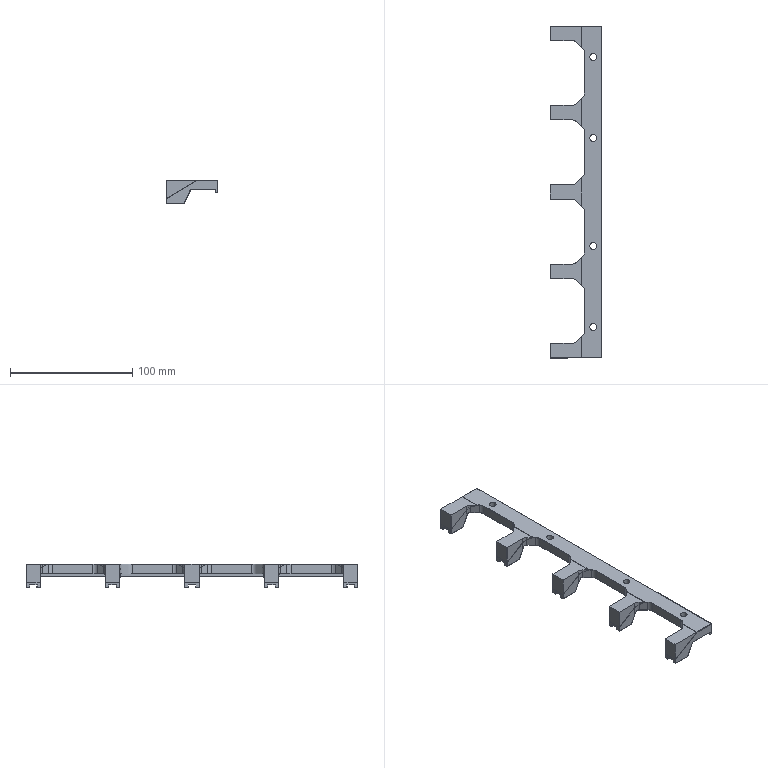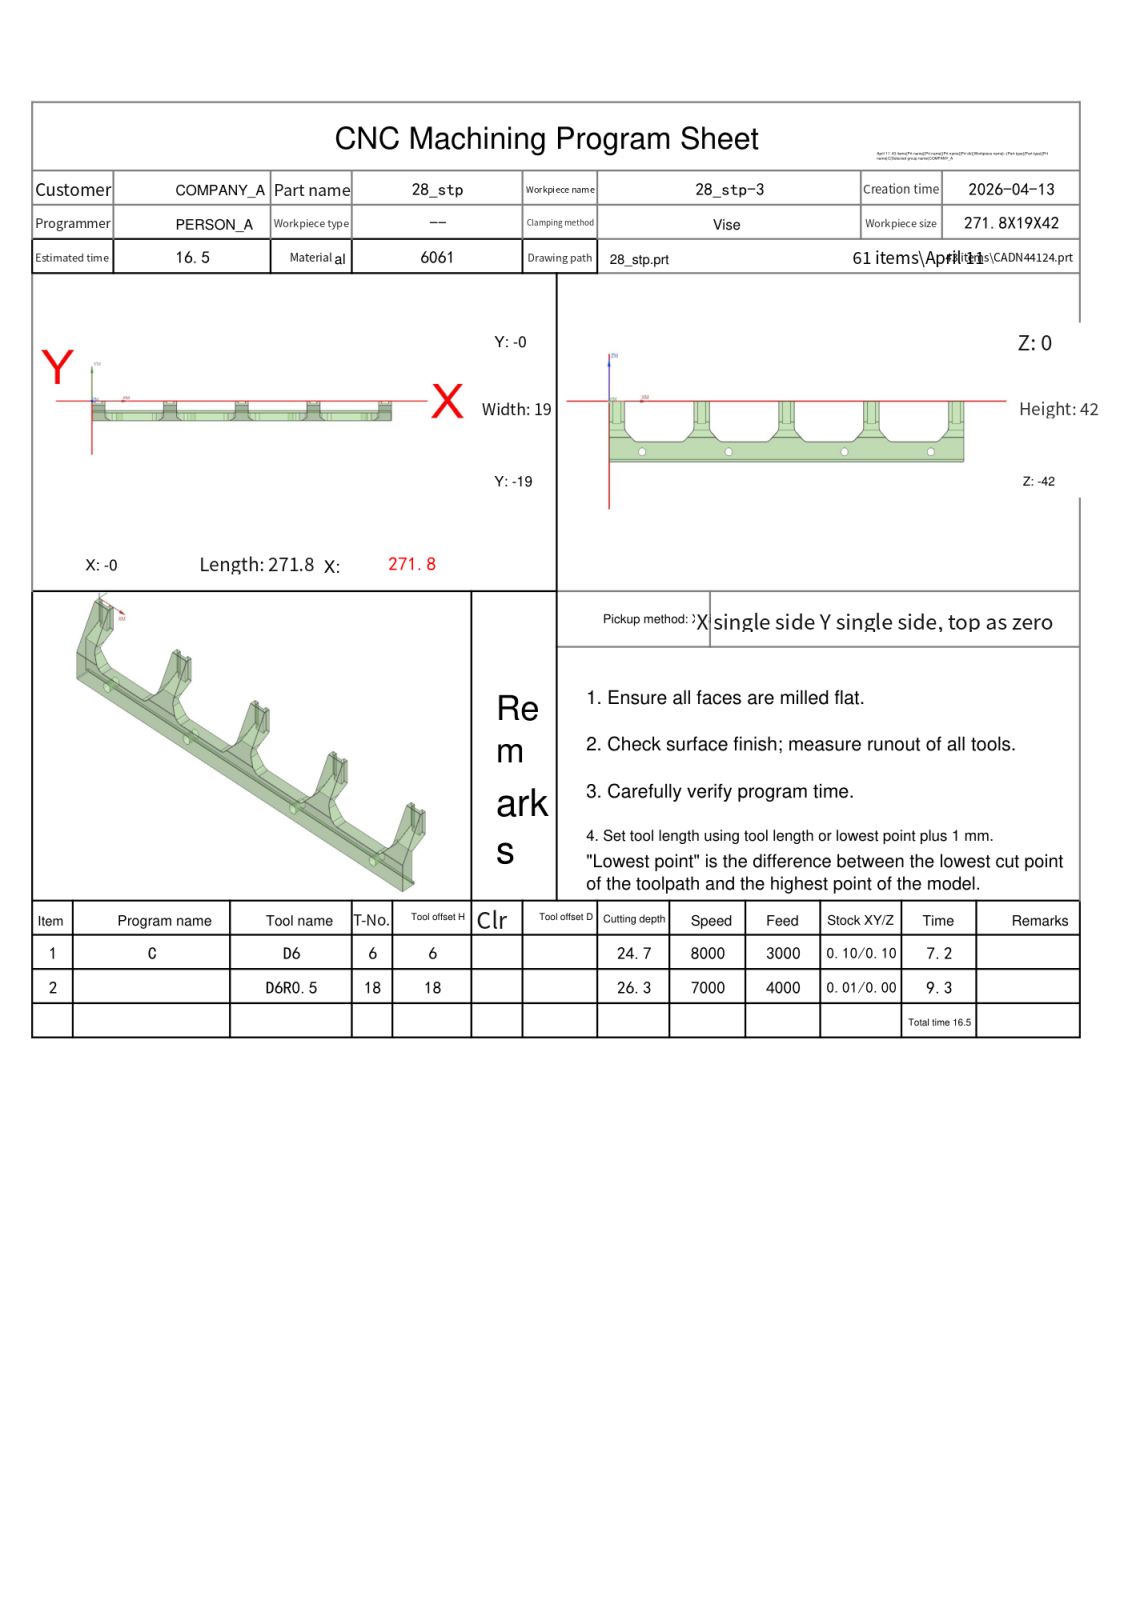NC program | NX | posted by the shop | part box 42 x 271.8 x 19 mm
Lines 8981 to 10169 of 25484:
N2 T18 M06
(D6R0.5  D=6. R=0.5 H=18 ce=0.01 di=0.00)
G00 G90 G54 X264.168 Y-6.651 M03 S7000
G43 H18 Z11.1
M08
Z1.113
G01 Z.613 F4000.
X259.69 Y-5.416
X258.972 Y-5.218
X258.804 Y-5.139
X258.651 Y-5.118 Z.595
X258.511 Y-5.071 Z.577
X258.381 Y-5.011 Z.559
G03 X260.049 Y-5.545 I1.668 J2.336
G01 X260.103
X260.241 Y-5.588 Z.533
X260.379 Y-5.628 Z.507
G02 X260.097 Y-5.641 I-.282 J3.036
X258.218 Y-4.993 I0.0 J3.049
G00 Z11.1
X17.341 Y-3.657
Z1.113
G01 Z.613
X12.763 Y-5.211
X12.436 Y-5.322
X12.366 Y-5.334
X12.217 Y-5.404 Z.599
X12.064 Y-5.461 Z.586
X11.91 Y-5.499 Z.572
X11.756 Y-5.527 Z.559
G03 X13.39 Y-5.009 I-.03 J2.93
G01 X13.505 Y-5.001 Z.533
X13.608 Y-4.976 Z.507
G02 X11.623 Y-5.635 I-1.985 J2.665
X11.423 Y-5.629 I0.0 J3.323
G00 Z11.1
X4.846 Y-5.95
Z1.113
G01 Z.613
X-.217 Y-5.414
G02 X-1.126 Y-5.134 I.26 J2.453
G01 X-1.278 Y-5.109 Z.595
X-1.417 Y-5.061 Z.577
X-1.548 Y-5.001 Z.559
G03 X.124 Y-5.546 I1.672 J2.294
G01 X.203 Y-5.545
X.325 Y-5.577 Z.542
X.447 Y-5.604 Z.524
X.569 Y-5.628 Z.507
G02 X.229 Y-5.646 I-.339 J3.2
X-1.737 Y-4.975 I0.0 J3.218
G01 X-1.81 Y-4.996 Z.458
G03 X.183 Y-5.717 I1.996 J2.4
G01 X2.073 Y-5.719
X11.093 Y-5.718
X11.682 Y-5.717
G03 X13.703 Y-4.991 I-.011 J3.206
G01 X13.771 Y-5.013 Z.409
G02 X11.657 Y-5.805 I-2.115 J2.43
G01 X2.073 Y-5.806
X.205 Y-5.802
G02 X-1.878 Y-5.016 I.007 J3.172
G01 X-1.946 Y-5.037 Z.359
G03 X.251 Y-5.887 I2.208 J2.441
G01 X2.073 Y-5.893
X11.642 Y-5.892
G03 X13.84 Y-5.036 I0.0 J3.253
G01 X13.915 Y-5.052 Z.31
G02 X11.62 Y-5.979 I-2.295 J2.379
G01 X2.073 Y-5.98
X.685 Y-5.975
X.228 Y-5.972
G02 X-1.701 Y-5.303 I.019 J3.169
G01 X-2.015 Y-5.059
X-2.085 Y-5.083 Z.261
X-1.396 Y-5.59
G03 X.309 Y-6.06 I1.705 J2.858
G01 X.338
X2.073 Y-6.067
X11.44 Y-6.066
X11.788 Y-6.06
G03 X13.302 Y-5.588 I-.055 J2.843
X13.993 Y-5.064 I-3.716 J5.62
G01 X14.071 Y-5.077 Z.212
X13.453 Y-5.555
G02 X11.704 Y-6.154 I-1.749 J2.258
G01 X1.379 Y-6.153
X.26 Y-6.148
G02 X-1.35 Y-5.687 I.014 J3.095
X-2.171 Y-5.084 I3.325 J5.394
G01 X-2.259 Y-5.085 Z.162
X-1.563 Y-5.618
G03 X.247 Y-6.236 I1.824 J2.383
G01 X1.379 Y-6.241
X11.667
G03 X13.528 Y-5.587 I0.0 J2.978
G01 X14.15 Y-5.09
X14.239 Y-5.093 Z.113
X14.216 Y-5.114
X13.522 Y-5.669
G02 X11.787 Y-6.323 I-1.874 J2.344
G01 X11.44 Y-6.328
X1.379 Y-6.329
X.257 Y-6.324
G02 X-1.603 Y-5.674 I.013 J3.024
G01 X-2.347 Y-5.087
X-2.436 Y-5.09 Z.064
X-1.563 Y-5.778
G03 X.256 Y-6.412 I1.829 J2.321
G01 X1.379 Y-6.416
X11.648 Y-6.414
X11.762 Y-6.411
G03 X13.295 Y-5.902 I-.064 J2.755
X14.367 Y-5.051 I-7.464 J10.497
G01 X14.491 Y-5.012 Z.017
G02 X13.354 Y-5.937 I-11.479 J12.943
X11.721 Y-6.496 I-1.685 J2.259
G01 X11.648 Y-6.497
X.261 Y-6.496
G02 X-1.558 Y-5.856 I0.0 J2.905
G01 X-2.437 Y-5.149
X-2.578 Y-5.025
X-2.677 Y-4.98 Z-.016
G03 X-2.195 Y-5.394 I6.378 J6.933
G01 X-1.532 Y-5.926
G03 X.256 Y-6.555 I1.789 J2.229
G01 X11.579 Y-6.556
X11.642 Y-6.557
G03 X13.315 Y-6.02 I0.0 J2.876
X14.576 Y-4.98 I-10.632 J14.176
G01 X14.637 Y-4.951 Z-.053
G02 X13.307 Y-6.082 I-8.368 J8.492
X11.718 Y-6.62 I-1.66 J2.287
G01 X.252
G02 X-1.506 Y-6.009 I.009 J2.86
G01 X-2.343 Y-5.316
G02 X-2.761 Y-4.93 I3.319 J4.01
G01 X-2.803 Y-4.925 Z-.098
G03 X-2.01 Y-5.666 I5.054 J4.614
G01 X-1.743 Y-5.882
X-1.596 Y-6.009
G03 X.256 Y-6.701 I1.875 J2.193
G01 X11.646
G03 X13.257 Y-6.185 I0.0 J2.771
X14.709 Y-4.915 I-5.715 J7.996
G01 X14.776 Y-4.872 Z-.145
G02 X13.817 Y-5.816 I-5.844 J4.98
G01 X13.479 Y-6.095
G02 X11.624 Y-6.785 I-1.911 J2.3
G01 X.276
G02 X-1.396 Y-6.231 I.005 J2.817
G01 X-1.679 Y-6.009
G02 X-2.826 Y-4.932 I4.857 J6.325
G01 X-2.849 Y-4.938 Z-.198
G03 X-1.338 Y-6.353 I6.547 J5.482
X.284 Y-6.869 I1.632 J2.321
G01 X11.613
G03 X13.453 Y-6.191 I-.023 J2.901
G01 X13.578 Y-6.088
G03 X14.85 Y-4.822 I-5.324 J6.62
G01 X14.91 Y-4.794 Z-.261
X14.216 Y-5.584
X14.136 Y-5.666
X13.63 Y-6.136
X13.462 Y-6.275
G02 X11.614 Y-6.938 I-1.848 J2.241
G01 X.282
G02 X-1.534 Y-6.295 I0.0 J2.886
X-2.877 Y-4.945 I5.583 J6.895
G01 X-2.907 Y-4.952 Z-.329
G03 X-1.963 Y-6.009 I14.585 J12.07
X.283 Y-6.99 I2.25 J2.09
G01 X11.614
G03 X13.861 Y-6.009 I-.001 J3.066
X14.911 Y-4.833 I-15.381 J14.784
G01 X14.912 Y-4.878 Z-.407
G02 X13.869 Y-6.076 I-37.077 J31.237
X11.691 Y-7.037 I-2.178 J1.987
G01 X11.684
X.209
G02 X-1.95 Y-6.095 I0.0 J2.948
G01 X-2.09 Y-5.945
X-2.94 Y-4.96
X-2.976 Y-4.969 Z-.488
X-2.229 Y-5.841
X-2.09 Y-6.003
G03 X.2 Y-7.086 I2.304 J1.908
G01 X11.7
G03 X13.983 Y-6.011 I-.028 J3.02
G01 X14.129 Y-5.841
X14.913 Y-4.926
X14.914 Y-4.974 Z-.572
X14.159 Y-5.856
X13.959 Y-6.089
G02 X11.7 Y-7.136 I-2.268 J1.933
G01 X.2
G02 X-2.059 Y-6.089 I.009 J2.98
G01 X-2.259 Y-5.856
X-3.012 Y-4.978
X-3.014 Y-5.025 Z-.657
X-2.259 Y-5.907
X-2.059 Y-6.141
G03 X.2 Y-7.188 I2.268 J1.933
G01 X11.7
G03 X13.959 Y-6.141 I-.009 J2.98
G01 X14.159 Y-5.907
X14.915 Y-5.025
Y-5.076 Z-.743
X14.159 Y-5.959
X13.959 Y-6.192
G02 X11.7 Y-7.239 I-2.268 J1.933
G01 X.2
G02 X-2.059 Y-6.192 I.009 J2.98
G01 X-2.259 Y-5.959
X-3.014 Y-5.075
Y-5.125 Z-.829
X-2.259 Y-6.01
X-2.059 Y-6.244
G03 X.2 Y-7.29 I2.268 J1.933
G01 X11.7
G03 X13.959 Y-6.244 I-.009 J2.98
G01 X14.159 Y-6.01
X14.916 Y-5.127
Y-5.178 Z-.915
X14.159 Y-6.062
X13.959 Y-6.295
G02 X11.7 Y-7.342 I-2.268 J1.933
G01 X.2
G02 X-2.059 Y-6.295 I.009 J2.98
G01 X-2.259 Y-6.062
X-2.893 Y-5.322
X-3.014 Y-5.177
X-3.015 Y-5.228 Z-1.
X-2.937 Y-5.322
X-2.259 Y-6.113
X-2.059 Y-6.346
G03 X.2 Y-7.393 I2.268 J1.933
G01 X11.7
G03 X13.959 Y-6.346 I-.009 J2.98
G01 X14.159 Y-6.113
X14.917 Y-5.229
Y-5.28 Z-1.086
X14.159 Y-6.165
X13.959 Y-6.398
G02 X11.7 Y-7.445 I-2.268 J1.933
G01 X.2
G02 X-2.059 Y-6.398 I.009 J2.98
G01 X-2.259 Y-6.165
X-2.982 Y-5.322
X-3.017 Y-5.279
X-3.018 Y-5.331 Z-1.172
X-2.259 Y-6.216
X-2.059 Y-6.449
G03 X.2 Y-7.496 I2.268 J1.933
G01 X11.7
G03 X13.959 Y-6.449 I-.009 J2.98
G01 X14.159 Y-6.216
X14.918 Y-5.331
Y-5.382 Z-1.258
X14.159 Y-6.268
X13.959 Y-6.501
G02 X11.7 Y-7.548 I-2.268 J1.933
G01 X.2
G02 X-2.059 Y-6.501 I.009 J2.98
G01 X-2.259 Y-6.268
X-3.017 Y-5.381
Y-5.431 Z-1.343
X-2.259 Y-6.319
X-2.059 Y-6.552
G03 X.2 Y-7.599 I2.268 J1.933
G01 X11.7
G03 X13.959 Y-6.552 I-.009 J2.98
G01 X14.159 Y-6.319
X14.918 Y-5.433
X14.919 Y-5.483 Z-1.429
X14.159 Y-6.37
X13.959 Y-6.604
G02 X11.7 Y-7.651 I-2.268 J1.933
G01 X.2
G02 X-2.059 Y-6.604 I.009 J2.98
G01 X-2.259 Y-6.37
X-3.017 Y-5.482
X-3.018 Y-5.533 Z-1.515
X-2.908 Y-5.666
X-2.259 Y-6.422
X-2.059 Y-6.655
G03 X.2 Y-7.702 I2.268 J1.933
G01 X11.7
G03 X13.959 Y-6.655 I-.009 J2.98
G01 X14.159 Y-6.422
X14.919 Y-5.534
X14.92 Y-5.585 Z-1.601
X14.159 Y-6.473
X13.959 Y-6.707
G02 X11.7 Y-7.754 I-2.268 J1.933
G01 X.2
G02 X-2.059 Y-6.707 I.009 J2.98
G01 X-2.259 Y-6.473
X-2.952 Y-5.666
X-3.019 Y-5.585
X-3.02 Y-5.636 Z-1.686
X-2.996 Y-5.666
X-2.259 Y-6.525
X-2.059 Y-6.758
G03 X.2 Y-7.805 I2.268 J1.933
G01 X11.7
G03 X13.959 Y-6.758 I-.009 J2.98
G01 X14.159 Y-6.525
X14.909 Y-5.65
X14.92 Y-5.636
X14.921 Y-5.687 Z-1.772
X14.159 Y-6.576
X13.959 Y-6.81
G02 X11.7 Y-7.856 I-2.268 J1.933
G01 X.2
G02 X-2.059 Y-6.81 I.009 J2.98
G01 X-2.259 Y-6.576
X-3.021 Y-5.687
X-3.02 Y-5.737 Z-1.858
X-2.259 Y-6.628
X-2.059 Y-6.861
G03 X.2 Y-7.908 I2.268 J1.933
G01 X11.7
G03 X13.959 Y-6.861 I-.009 J2.98
G01 X14.159 Y-6.628
X14.921 Y-5.738
Y-5.789 Z-1.944
X14.159 Y-6.679
X13.959 Y-6.912
G02 X11.7 Y-7.959 I-2.268 J1.933
G01 X.2
G02 X-2.059 Y-6.912 I.009 J2.98
G01 X-2.259 Y-6.679
X-3.02 Y-5.788
Y-5.839 Z-2.029
X-2.878 Y-6.009
X-2.259 Y-6.731
X-2.059 Y-6.964
G03 X.2 Y-8.011 I2.268 J1.933
G01 X11.7
G03 X13.959 Y-6.964 I-.009 J2.98
G01 X14.159 Y-6.731
X14.922 Y-5.84
Y-5.891 Z-2.115
X14.159 Y-6.782
X13.959 Y-7.015
G02 X11.7 Y-8.062 I-2.268 J1.933
G01 X.2
G02 X-2.059 Y-7.015 I.009 J2.98
G01 X-2.259 Y-6.782
X-2.922 Y-6.009
X-3.021 Y-5.89
X-3.022 Y-5.941 Z-2.201
X-2.966 Y-6.009
X-2.259 Y-6.833
X-2.059 Y-7.067
G03 X.2 Y-8.114 I2.268 J1.933
G01 X11.7
G03 X13.959 Y-7.067 I-.009 J2.98
G01 X14.159 Y-6.833
X14.909 Y-5.959
X14.922 Y-5.941
X14.923 Y-5.992 Z-2.287
X14.91 Y-6.009
X14.159 Y-6.885
X13.959 Y-7.118
G02 X11.7 Y-8.165 I-2.268 J1.933
G01 X.2
G02 X-2.059 Y-7.118 I.009 J2.98
G01 X-2.259 Y-6.885
X-3.023 Y-5.993
Y-6.044 Z-2.372
X-2.259 Y-6.936
X-2.059 Y-7.17
G03 X.2 Y-8.217 I2.268 J1.933
G01 X11.7
G03 X13.959 Y-7.17 I-.009 J2.98
G01 X14.159 Y-6.936
X14.924 Y-6.044
Y-6.095 Z-2.458
X14.159 Y-6.988
X13.959 Y-7.221
G02 X11.7 Y-8.268 I-2.268 J1.933
G01 X.2
G02 X-2.059 Y-7.221 I.009 J2.98
G01 X-2.259 Y-6.988
X-3.023 Y-6.094
Y-6.145 Z-2.544
X-2.259 Y-7.039
X-2.059 Y-7.273
G03 X.2 Y-8.319 I2.268 J1.933
G01 X11.7
G03 X13.959 Y-7.273 I-.009 J2.98
G01 X14.159 Y-7.039
X14.924 Y-6.146
X14.925 Y-6.197 Z-2.63
X14.159 Y-7.091
X13.959 Y-7.324
G02 X11.7 Y-8.371 I-2.268 J1.933
G01 X.2
G02 X-2.059 Y-7.324 I.009 J2.98
G01 X-2.259 Y-7.091
X-2.892 Y-6.353
X-3.023 Y-6.196
X-3.024 Y-6.247 Z-2.715
X-2.936 Y-6.353
X-2.259 Y-7.142
X-2.059 Y-7.375
G03 X.2 Y-8.422 I2.268 J1.933
G01 X11.7
G03 X13.959 Y-7.375 I-.009 J2.98
G01 X14.159 Y-7.142
X14.909 Y-6.267
X14.925 Y-6.247
Y-6.298 Z-2.801
X14.909 Y-6.319
X14.159 Y-7.194
X13.959 Y-7.427
G02 X11.7 Y-8.474 I-2.268 J1.933
G01 X.2
G02 X-2.059 Y-7.427 I.009 J2.98
G01 X-2.259 Y-7.194
X-2.98 Y-6.353
X-3.025 Y-6.299
X-3.026 Y-6.351 Z-2.887
X-2.259 Y-7.245
X-2.059 Y-7.478
G03 X.2 Y-8.525 I2.268 J1.933
G01 X11.7
G03 X13.959 Y-7.478 I-.009 J2.98
G01 X14.159 Y-7.245
X14.927 Y-6.35
X14.926 Y-6.401 Z-2.973
X14.159 Y-7.297
X13.959 Y-7.53
G02 X11.7 Y-8.577 I-2.268 J1.933
G01 X.2
G02 X-2.059 Y-7.53 I.009 J2.98
G01 X-2.259 Y-7.297
X-3.026 Y-6.401
X-3.025 Y-6.451 Z-3.058
X-2.259 Y-7.348
X-2.059 Y-7.581
G03 X.2 Y-8.628 I2.268 J1.933
G01 X11.7
G03 X13.959 Y-7.581 I-.009 J2.98
G01 X14.159 Y-7.348
X14.927 Y-6.452
Y-6.503 Z-3.144
X14.909 Y-6.525
X14.159 Y-7.399
X13.959 Y-7.633
G02 X11.7 Y-8.68 I-2.268 J1.933
G01 X.2
G02 X-2.059 Y-7.633 I.009 J2.98
G01 X-2.259 Y-7.399
X-3.025 Y-6.502
X-3.026 Y-6.553 Z-3.23
X-2.906 Y-6.696
X-2.259 Y-7.451
X-2.059 Y-7.684
G03 X.2 Y-8.731 I2.268 J1.933
G01 X11.7
G03 X13.959 Y-7.684 I-.009 J2.98
G01 X14.159 Y-7.451
X14.909 Y-6.576
X14.927 Y-6.554
Y-6.605 Z-3.316
X14.909 Y-6.627
X14.159 Y-7.502
X13.959 Y-7.736
G02 X11.7 Y-8.783 I-2.268 J1.933
G01 X.2
G02 X-2.059 Y-7.736 I.009 J2.98
G01 X-2.259 Y-7.502
X-2.95 Y-6.696
X-3.027 Y-6.605
X-3.028 Y-6.656 Z-3.401
X-2.994 Y-6.696
X-2.259 Y-7.554
X-2.059 Y-7.787
G03 X.2 Y-8.834 I2.268 J1.933
G01 X11.7
G03 X13.959 Y-7.787 I-.009 J2.98
G01 X14.159 Y-7.554
X14.909 Y-6.679
X14.927 Y-6.656
X14.929 Y-6.707 Z-3.487
X14.159 Y-7.605
X13.959 Y-7.839
G02 X11.7 Y-8.885 I-2.268 J1.933
G01 X.2
G02 X-2.059 Y-7.839 I.009 J2.98
G01 X-2.259 Y-7.605
X-3.028 Y-6.708
Y-6.758 Z-3.573
X-2.259 Y-7.657
X-2.059 Y-7.89
G03 X.2 Y-8.937 I2.268 J1.933
G01 X11.7
G03 X13.959 Y-7.89 I-.009 J2.98
G01 X14.159 Y-7.657
X14.909 Y-6.782
X14.928 Y-6.758
X14.929 Y-6.809 Z-3.659
X14.909 Y-6.833
X14.159 Y-7.708
X13.959 Y-7.941
G02 X11.7 Y-8.988 I-2.268 J1.933
G01 X.2
G02 X-2.059 Y-7.941 I.009 J2.98
G01 X-2.259 Y-7.708
X-3.027 Y-6.808
X-3.028 Y-6.86 Z-3.744
X-2.876 Y-7.04
X-2.259 Y-7.76
X-2.059 Y-7.993
G03 X.2 Y-9.04 I2.268 J1.933
G01 X11.7
G03 X13.959 Y-7.993 I-.009 J2.98
G01 X14.159 Y-7.76
X14.909 Y-6.885
X14.929 Y-6.86
Y-6.911 Z-3.83
X14.909 Y-6.936
X14.159 Y-7.811
X13.959 Y-8.044
G02 X11.7 Y-9.091 I-2.268 J1.933
G01 X.2
G02 X-2.059 Y-8.044 I.009 J2.98
G01 X-2.259 Y-7.811
X-2.92 Y-7.04
X-3.028 Y-6.911
X-3.029 Y-6.962 Z-3.916
X-2.965 Y-7.04
X-2.259 Y-7.862
X-2.059 Y-8.096
G03 X.2 Y-9.143 I2.268 J1.933
G01 X11.7
G03 X13.959 Y-8.096 I-.009 J2.98
G01 X14.159 Y-7.862
X14.909 Y-6.988
X14.929 Y-6.962
Y-7.013 Z-4.002
X14.909 Y-7.039
X14.159 Y-7.914
X13.959 Y-8.147
G02 X11.7 Y-9.194 I-2.268 J1.933
G01 X.2
G02 X-2.059 Y-8.147 I.009 J2.98
G01 X-2.259 Y-7.914
X-3.009 Y-7.04
X-3.03 Y-7.014
Y-7.065 Z-4.087
X-2.259 Y-7.965
X-2.059 Y-8.199
G03 X.2 Y-9.246 I2.268 J1.933
G01 X11.7
G03 X13.959 Y-8.199 I-.009 J2.98
G01 X14.159 Y-7.965
X14.909 Y-7.091
X14.931 Y-7.065
Y-7.116 Z-4.173
X14.909 Y-7.142
X14.159 Y-8.017
X13.959 Y-8.25
G02 X11.7 Y-9.297 I-2.268 J1.933
G01 X.2
G02 X-2.059 Y-8.25 I.009 J2.98
G01 X-2.259 Y-8.017
X-3.03 Y-7.116
X-3.029 Y-7.166 Z-4.259
X-2.259 Y-8.068
X-2.059 Y-8.302
G03 X.2 Y-9.348 I2.268 J1.933
G01 X11.7
G03 X13.959 Y-8.302 I-.009 J2.98
G01 X14.159 Y-8.068
X14.909 Y-7.193
X14.931 Y-7.167
Y-7.218 Z-4.345
X14.909 Y-7.245
X14.159 Y-8.12
X13.959 Y-8.353
G02 X11.7 Y-9.4 I-2.268 J1.933
G01 X.2
G02 X-2.059 Y-8.353 I.009 J2.98
G01 X-2.259 Y-8.12
X-2.891 Y-7.384
X-3.03 Y-7.218
Y-7.269 Z-4.43
X-2.935 Y-7.384
X-2.259 Y-8.171
X-2.059 Y-8.404
G03 X.2 Y-9.451 I2.268 J1.933
G01 X11.7
G03 X13.959 Y-8.404 I-.009 J2.98
G01 X14.159 Y-8.171
X14.909 Y-7.296
X14.931 Y-7.269
Y-7.32 Z-4.516
X14.909 Y-7.348
X14.159 Y-8.223
X13.959 Y-8.456
G02 X11.7 Y-9.503 I-2.268 J1.933
G01 X.2
G02 X-2.059 Y-8.456 I.009 J2.98
G01 X-2.259 Y-8.223
X-2.979 Y-7.384
X-3.031 Y-7.321
X-3.032 Y-7.372 Z-4.602
X-2.259 Y-8.274
X-2.059 Y-8.507
G03 X.2 Y-9.554 I2.268 J1.933
G01 X11.7
G03 X13.959 Y-8.507 I-.009 J2.98
G01 X14.159 Y-8.274
X14.923 Y-7.384
X14.932 Y-7.372
Y-7.423 Z-4.688
X14.909 Y-7.451
X14.159 Y-8.326
X13.959 Y-8.559
G02 X11.7 Y-9.606 I-2.268 J1.933
G01 X.2
G02 X-2.059 Y-8.559 I.009 J2.98
G01 X-2.259 Y-8.326
X-3.032 Y-7.423
X-3.031 Y-7.474 Z-4.773
X-2.259 Y-8.377
X-2.059 Y-8.61
G03 X.2 Y-9.657 I2.268 J1.933
G01 X11.7
G03 X13.959 Y-8.61 I-.009 J2.98
G01 X14.159 Y-8.377
X14.909 Y-7.502
X14.932 Y-7.474
Y-7.525 Z-4.859
X14.909 Y-7.554
X14.159 Y-8.428
X13.959 Y-8.662
G02 X11.7 Y-9.709 I-2.268 J1.933
G01 X.2
G02 X-2.059 Y-8.662 I.009 J2.98
G01 X-2.259 Y-8.428
X-3.031 Y-7.525
Y-7.576 Z-4.945
X-2.905 Y-7.727
X-2.259 Y-8.48
X-2.059 Y-8.713
G03 X.2 Y-9.76 I2.268 J1.933
G01 X11.7
G03 X13.959 Y-8.713 I-.009 J2.98
G01 X14.159 Y-8.48
X14.909 Y-7.605
X14.932 Y-7.576
Y-7.627 Z-5.031
X14.909 Y-7.656
X14.159 Y-8.531
X13.959 Y-8.765
G02 X11.7 Y-9.811 I-2.268 J1.933
G01 X.2
G02 X-2.059 Y-8.765 I.009 J2.98
G01 X-2.259 Y-8.531
X-2.949 Y-7.727
X-3.032 Y-7.628
Y-7.679 Z-5.116
X-2.993 Y-7.727
X-2.259 Y-8.583
X-2.059 Y-8.816
G03 X.2 Y-9.863 I2.268 J1.933
G01 X11.7
G03 X13.959 Y-8.816 I-.009 J2.98
G01 X14.159 Y-8.583
X14.909 Y-7.708
X14.932 Y-7.678
X14.934 Y-7.731 Z-5.202
X14.159 Y-8.634
X13.959 Y-8.868
G02 X11.7 Y-9.914 I-2.268 J1.933
G01 X.2
G02 X-2.059 Y-8.868 I.009 J2.98
G01 X-2.259 Y-8.634
X-3.033 Y-7.731
X-3.032 Y-7.782 Z-5.288
X-2.259 Y-8.686
X-2.059 Y-8.919
G03 X.2 Y-9.966 I2.268 J1.933
G01 X11.7
G03 X13.959 Y-8.919 I-.009 J2.98
G01 X14.159 Y-8.686
X14.909 Y-7.811
X14.933 Y-7.782
Y-7.833 Z-5.374
X14.909 Y-7.862
X14.159 Y-8.737
X13.959 Y-8.97
G02 X11.7 Y-10.017 I-2.268 J1.933
G01 X.2
G02 X-2.059 Y-8.97 I.009 J2.98
G01 X-2.259 Y-8.737
X-3.032 Y-7.832
Y-7.884 Z-5.459
X-2.259 Y-8.789
X-2.059 Y-9.022
G03 X.2 Y-10.069 I2.268 J1.933
G01 X11.7
G03 X13.959 Y-9.022 I-.009 J2.98
G01 X14.159 Y-8.789
X14.909 Y-7.914
X14.933 Y-7.884
Y-7.935 Z-5.545
X14.909 Y-7.965
X14.159 Y-8.84
X13.959 Y-9.073
G02 X11.7 Y-10.12 I-2.268 J1.933
G01 X.2
G02 X-2.059 Y-9.073 I.009 J2.98
G01 X-2.259 Y-8.84
X-2.919 Y-8.071
X-3.032 Y-7.935
X-3.033 Y-7.987 Z-5.631
X-2.963 Y-8.071
X-2.259 Y-8.891
X-2.059 Y-9.125
G03 X.2 Y-10.172 I2.268 J1.933
G01 X11.7
G03 X13.959 Y-9.125 I-.009 J2.98
G01 X14.159 Y-8.891
X14.909 Y-8.017
X14.933 Y-7.986
Y-8.037 Z-5.717
X14.909 Y-8.068
X14.159 Y-8.943
X13.959 Y-9.176
G02 X11.7 Y-10.223 I-2.268 J1.933
G01 X.2
G02 X-2.059 Y-9.176 I.009 J2.98
G01 X-2.259 Y-8.943
X-3.007 Y-8.071
X-3.034 Y-8.039
Y-8.09 Z-5.802
X-2.259 Y-8.994
X-2.059 Y-9.228
G03 X.2 Y-10.275 I2.268 J1.933
G01 X11.7
G03 X13.959 Y-9.228 I-.009 J2.98
G01 X14.159 Y-8.994
X14.934 Y-8.089
Y-8.141 Z-5.888
X14.909 Y-8.171
X14.159 Y-9.046
X13.959 Y-9.279
G02 X11.7 Y-10.326 I-2.268 J1.933
G01 X.2
G02 X-2.059 Y-9.279 I.009 J2.98
G01 X-2.259 Y-9.046
X-3.033 Y-8.141
Y-8.191 Z-5.974
X-2.259 Y-9.097
X-2.059 Y-9.331
G03 X.2 Y-10.377 I2.268 J1.933
G01 X11.7
G03 X13.959 Y-9.331 I-.009 J2.98
G01 X14.159 Y-9.097
X14.909 Y-8.222
X14.934 Y-8.192
Y-8.243 Z-6.06
X14.909 Y-8.274
X14.159 Y-9.149
X13.959 Y-9.382
G02 X11.7 Y-10.429 I-2.268 J1.933
G01 X.2
G02 X-2.059 Y-9.382 I.009 J2.98
G01 X-2.259 Y-9.149
X-2.889 Y-8.414
X-3.033 Y-8.243
Y-8.294 Z-6.145
X-2.933 Y-8.414
X-2.259 Y-9.2
X-2.059 Y-9.433
G03 X.2 Y-10.48 I2.268 J1.933
G01 X11.7
G03 X13.959 Y-9.433 I-.009 J2.98
G01 X14.159 Y-9.2
X14.909 Y-8.325
X14.934 Y-8.294
X14.933 Y-8.345 Z-6.231
X14.909 Y-8.377
X14.159 Y-9.252
X13.959 Y-9.485
G02 X11.7 Y-10.532 I-2.268 J1.933
G01 X.2
G02 X-2.059 Y-9.485 I.009 J2.98
G01 X-2.259 Y-9.252
X-2.977 Y-8.414
X-3.034 Y-8.346
X-3.035 Y-8.398 Z-6.317
X-2.259 Y-9.303
X-2.059 Y-9.536
G03 X.2 Y-10.583 I2.268 J1.933
G01 X11.7
G03 X13.959 Y-9.536 I-.009 J2.98
G01 X14.159 Y-9.303
X14.921 Y-8.414
X14.934 Y-8.397
X14.935 Y-8.449 Z-6.403
X14.909 Y-8.48
X14.159 Y-9.355
X13.959 Y-9.588
G02 X11.7 Y-10.635 I-2.268 J1.933
G01 X.2
G02 X-2.059 Y-9.588 I.009 J2.98
G01 X-2.259 Y-9.355
X-3.034 Y-8.449
Y-8.5 Z-6.488
X-2.259 Y-9.406
X-2.059 Y-9.639
G03 X.2 Y-10.686 I2.268 J1.933
G01 X11.7
G03 X13.959 Y-9.639 I-.009 J2.98
G01 X14.159 Y-9.406
X14.909 Y-8.531
X14.934 Y-8.5
Y-8.551 Z-6.574
X14.909 Y-8.583
X14.159 Y-9.457
X13.959 Y-9.691
G02 X11.7 Y-10.738 I-2.268 J1.933
G01 X.2
G02 X-2.059 Y-9.691 I.009 J2.98
G01 X-2.259 Y-9.457
X-3.034 Y-8.551
Y-8.602 Z-6.66
X-2.903 Y-8.758
X-2.259 Y-9.509
X-2.059 Y-9.742
G03 X.2 Y-10.789 I2.268 J1.933
G01 X11.7
G03 X13.959 Y-9.742 I-.009 J2.98
G01 X14.159 Y-9.509
X14.909 Y-8.634
X14.934 Y-8.603
Y-8.654 Z-6.746
X14.909 Y-8.685
X14.159 Y-9.56
X13.959 Y-9.794
G02 X11.7 Y-10.84 I-2.268 J1.933
G01 X.2
G02 X-2.059 Y-9.794 I.009 J2.98
G01 X-2.259 Y-9.56
X-2.947 Y-8.758
X-3.034 Y-8.654
X-3.035 Y-8.706 Z-6.831
X-2.991 Y-8.758
X-2.259 Y-9.612
X-2.059 Y-9.845
G03 X.2 Y-10.892 I2.268 J1.933
G01 X11.7
G03 X13.959 Y-9.845 I-.009 J2.98
G01 X14.159 Y-9.612
X14.909 Y-8.737
X14.934 Y-8.705
X14.936 Y-8.758 Z-6.917
X14.159 Y-9.663
X13.959 Y-9.896
G02 X11.7 Y-10.943 I-2.268 J1.933
G01 X.2
G02 X-2.059 Y-9.896 I.009 J2.98
G01 X-2.259 Y-9.663
X-3.036 Y-8.758
X-3.035 Y-8.808 Z-7.003
X-2.259 Y-9.715
X-2.059 Y-9.948
G03 X.2 Y-10.995 I2.268 J1.933
G01 X11.7
G03 X13.959 Y-9.948 I-.009 J2.98
G01 X14.159 Y-9.715
X14.909 Y-8.84
X14.935 Y-8.808
Y-8.86 Z-7.089
X14.909 Y-8.891
X14.159 Y-9.766
X13.959 Y-9.999
G02 X11.7 Y-11.046 I-2.268 J1.933
G01 X.2
G02 X-2.059 Y-9.999 I.009 J2.98
G01 X-2.259 Y-9.766
X-3.034 Y-8.859
Y-8.91 Z-7.174
X-2.259 Y-9.818
X-2.059 Y-10.051
G03 X.2 Y-11.098 I2.268 J1.933
G01 X11.7
G03 X13.959 Y-10.051 I-.009 J2.98
G01 X14.159 Y-9.818
X14.909 Y-8.943
X14.935 Y-8.911
Y-8.962 Z-7.26
X14.909 Y-8.994
X14.159 Y-9.869
X13.959 Y-10.102
G02 X11.7 Y-11.149 I-2.268 J1.933
G01 X.2
G02 X-2.059 Y-10.102 I.009 J2.98
G01 X-2.259 Y-9.869
X-2.917 Y-9.101
X-3.034 Y-8.962
X-3.035 Y-9.014 Z-7.346
X-2.962 Y-9.101
X-2.259 Y-9.92
X-2.059 Y-10.154
G03 X.2 Y-11.201 I2.268 J1.933
G01 X11.7
G03 X13.959 Y-10.154 I-.009 J2.98
G01 X14.159 Y-9.92
X14.909 Y-9.046
X14.934 Y-9.013
Y-9.064 Z-7.432
X14.909 Y-9.097
X14.159 Y-9.972
X13.959 Y-10.205
G02 X11.7 Y-11.252 I-2.268 J1.933
G01 X.2
G02 X-2.059 Y-10.205 I.009 J2.98
G01 X-2.259 Y-9.972
X-3.006 Y-9.101
X-3.035 Y-9.065
X-3.036 Y-9.117 Z-7.517
X-2.259 Y-10.023
X-2.059 Y-10.257
G03 X.2 Y-11.304 I2.268 J1.933
G01 X11.7
G03 X13.959 Y-10.257 I-.009 J2.98
G01 X14.159 Y-10.023
X14.936 Y-9.117
X14.935 Y-9.168 Z-7.603
X14.909 Y-9.2
X14.159 Y-10.075
X13.959 Y-10.308
G02 X11.7 Y-11.355 I-2.268 J1.933
G01 X.2
G02 X-2.059 Y-10.308 I.009 J2.98
G01 X-2.259 Y-10.075
X-3.035 Y-9.168
X-3.034 Y-9.219 Z-7.689
X-2.259 Y-10.126
X-2.059 Y-10.36
G03 X.2 Y-11.406 I2.268 J1.933
G01 X11.7
G03 X13.959 Y-10.36 I-.009 J2.98
G01 X14.159 Y-10.126
X14.909 Y-9.251
X14.935 Y-9.219
Y-9.271 Z-7.775
X14.909 Y-9.303
X14.159 Y-10.178
X13.959 Y-10.411
G02 X11.7 Y-11.458 I-2.268 J1.933
G01 X.2
G02 X-2.059 Y-10.411 I.009 J2.98
G01 X-2.259 Y-10.178
X-2.888 Y-9.445
X-3.035 Y-9.27
Y-9.322 Z-7.86
X-2.932 Y-9.445
X-2.259 Y-10.229
X-2.059 Y-10.462
G03 X.2 Y-11.509 I2.268 J1.933
G01 X11.7
G03 X13.959 Y-10.462 I-.009 J2.98
G01 X14.159 Y-10.229
X14.909 Y-9.354
X14.935 Y-9.322
X14.934 Y-9.373 Z-7.946
X14.909 Y-9.406
X14.159 Y-10.281
X13.959 Y-10.514
G02 X11.7 Y-11.561 I-2.268 J1.933
G01 X.2
G02 X-2.059 Y-10.514 I.009 J2.98
G01 X-2.259 Y-10.281
X-2.976 Y-9.445
X-3.035 Y-9.374
X-3.036 Y-9.426 Z-8.032
X-2.259 Y-10.332
X-2.059 Y-10.565
G03 X.2 Y-11.612 I2.268 J1.933
G01 X11.7
G03 X13.959 Y-10.565 I-.009 J2.98
G01 X14.159 Y-10.332
X14.92 Y-9.445
X14.935 Y-9.425
X14.936 Y-9.477 Z-8.118
X14.909 Y-9.509
X14.159 Y-10.384
X13.959 Y-10.617
G02 X11.7 Y-11.664 I-2.268 J1.933
G01 X.2
G02 X-2.059 Y-10.617 I.009 J2.98
G01 X-2.259 Y-10.384
X-3.036 Y-9.477
X-3.035 Y-9.527 Z-8.203
X-2.259 Y-10.435
X-2.059 Y-10.668
G03 X.2 Y-11.715 I2.268 J1.933
G01 X11.7
G03 X13.959 Y-10.668 I-.009 J2.98
G01 X14.159 Y-10.435
X14.909 Y-9.56
X14.935 Y-9.528
Y-9.579 Z-8.289
X14.909 Y-9.612
X14.159 Y-10.486
X13.959 Y-10.72
G02 X11.7 Y-11.767 I-2.268 J1.933
G01 X.2
G02 X-2.059 Y-10.72 I.009 J2.98
G01 X-2.259 Y-10.486
X-3.035 Y-9.579
Y-9.63 Z-8.375
X-2.902 Y-9.789
X-2.259 Y-10.538
X-2.059 Y-10.771
G03 X.2 Y-11.818 I2.268 J1.933
G01 X11.7
G03 X13.959 Y-10.771 I-.009 J2.98
G01 X14.159 Y-10.538
X14.909 Y-9.663
X14.935 Y-9.631
Y-9.682 Z-8.461
X14.909 Y-9.714
X14.159 Y-10.589
X13.959 Y-10.823
G02 X11.7 Y-11.869 I-2.268 J1.933
G01 X.2
G02 X-2.059 Y-10.823 I.009 J2.98
G01 X-2.259 Y-10.589
X-2.946 Y-9.789
X-3.035 Y-9.682
X-3.036 Y-9.734 Z-8.546
X-2.99 Y-9.789
X-2.259 Y-10.641
X-2.059 Y-10.874
G03 X.2 Y-11.921 I2.268 J1.933
G01 X11.7
G03 X13.959 Y-10.874 I-.009 J2.98
G01 X14.159 Y-10.641
X14.909 Y-9.766
X14.935 Y-9.733
X14.936 Y-9.786 Z-8.632
X14.159 Y-10.692
X13.959 Y-10.925
G02 X11.7 Y-11.972 I-2.268 J1.933
G01 X.2
G02 X-2.059 Y-10.925 I.009 J2.98
G01 X-2.259 Y-10.692
X-3.036 Y-9.786
Y-9.836 Z-8.718
X-2.259 Y-10.744
X-2.059 Y-10.977
G03 X.2 Y-12.024 I2.268 J1.933
G01 X11.7
G03 X13.959 Y-10.977 I-.009 J2.98
G01 X14.159 Y-10.744
X14.909 Y-9.869
X14.936 Y-9.837
Y-9.888 Z-8.804
X14.909 Y-9.92
X14.159 Y-10.795
X13.959 Y-11.028
G02 X11.7 Y-12.075 I-2.268 J1.933
G01 X.2
G02 X-2.059 Y-11.028 I.009 J2.98
G01 X-2.259 Y-10.795
X-3.035 Y-9.887
Y-9.939 Z-8.889
X-2.259 Y-10.847
X-2.059 Y-11.08
G03 X.2 Y-12.127 I2.268 J1.933
G01 X11.7
G03 X13.959 Y-11.08 I-.009 J2.98
G01 X14.159 Y-10.847
X14.909 Y-9.972
X14.935 Y-9.939
Y-9.991 Z-8.975
X14.909 Y-10.023
X14.159 Y-10.898
X13.959 Y-11.131
G02 X11.7 Y-12.178 I-2.268 J1.933
G01 X.2
G02 X-2.059 Y-11.131 I.009 J2.98
G01 X-2.259 Y-10.898
X-2.916 Y-10.132
X-3.035 Y-9.99
Y-10.042 Z-9.061
X-2.96 Y-10.132
X-2.259 Y-10.949
X-2.059 Y-11.183
G03 X.2 Y-12.23 I2.268 J1.933
G01 X11.7
G03 X13.959 Y-11.183 I-.009 J2.98
G01 X14.159 Y-10.949
X14.909 Y-10.075
X14.935 Y-10.042
X14.934 Y-10.093 Z-9.147
X14.909 Y-10.126
X14.159 Y-11.001
X13.959 Y-11.234
G02 X11.7 Y-12.281 I-2.268 J1.933
G01 X.2
G02 X-2.059 Y-11.234 I.009 J2.98
G01 X-2.259 Y-11.001
X-3.004 Y-10.132
X-3.036 Y-10.094
Y-10.145 Z-9.232
X-2.259 Y-11.052
X-2.059 Y-11.286
G03 X.2 Y-12.333 I2.268 J1.933
G01 X11.7
G03 X13.959 Y-11.286 I-.009 J2.98
G01 X14.159 Y-11.052
X14.936 Y-10.146
Y-10.197 Z-9.318
X14.909 Y-10.229
X14.159 Y-11.104
X13.959 Y-11.337
G02 X11.7 Y-12.384 I-2.268 J1.933
G01 X.2
G02 X-2.059 Y-11.337 I.009 J2.98
G01 X-2.259 Y-11.104
X-3.035 Y-10.196
Y-10.247 Z-9.404
X-2.259 Y-11.155
X-2.059 Y-11.389
G03 X.2 Y-12.435 I2.268 J1.933
G01 X11.7
G03 X13.959 Y-11.389 I-.009 J2.98
G01 X14.159 Y-11.155
X14.909 Y-10.28
X14.936 Y-10.248
X14.935 Y-10.299 Z-9.49
X14.909 Y-10.332
X14.159 Y-11.207
X13.959 Y-11.44
G02 X11.7 Y-12.487 I-2.268 J1.933
G01 X.2
G02 X-2.059 Y-11.44 I.009 J2.98
G01 X-2.259 Y-11.207
X-2.886 Y-10.476
X-3.035 Y-10.299
Y-10.35 Z-9.575
X-2.93 Y-10.476
X-2.259 Y-11.258
X-2.059 Y-11.491
G03 X.2 Y-12.538 I2.268 J1.933
G01 X11.7
G03 X13.959 Y-11.491 I-.009 J2.98
G01 X14.159 Y-11.258
X14.909 Y-10.383
X14.935 Y-10.351
Y-10.402 Z-9.661
X14.909 Y-10.435
X14.159 Y-11.31
X13.959 Y-11.543
G02 X11.7 Y-12.59 I-2.268 J1.933
G01 X.2
G02 X-2.059 Y-11.543 I.009 J2.98
G01 X-2.259 Y-11.31
X-2.974 Y-10.476
X-3.036 Y-10.402
Y-10.454 Z-9.747
X-2.259 Y-11.361
X-2.059 Y-11.594
G03 X.2 Y-12.641 I2.268 J1.933
G01 X11.7
G03 X13.959 Y-11.594 I-.009 J2.98
G01 X14.159 Y-11.361
X14.918 Y-10.476
X14.935 Y-10.453
X14.936 Y-10.506 Z-9.833
X14.909 Y-10.538
X14.159 Y-11.413
X13.959 Y-11.646
G02 X11.7 Y-12.693 I-2.268 J1.933
G01 X.2
G02 X-2.059 Y-11.646 I.009 J2.98
G01 X-2.259 Y-11.413
X-3.036 Y-10.505